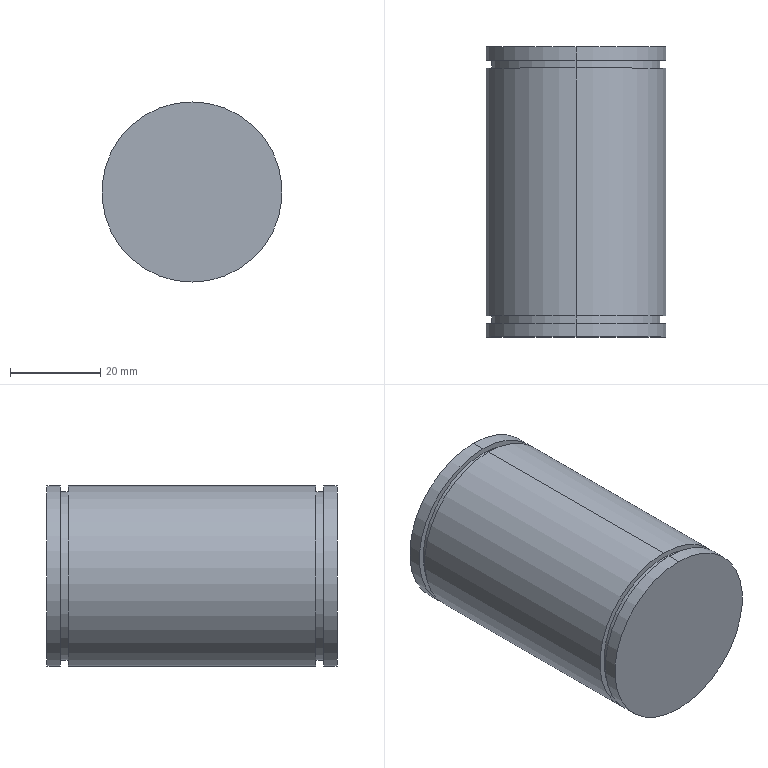Part | SolidWorks | features Extrusion 1, MirrorPattern 1, RevCut 1 | 1 solid | 16 faces | box 40 x 64.4 x 40 mm | volume 80410 mm3 | cylinder 10 | plane 6 | commonest cylinder face diameters 40 x6 37.5 x4
STEP:
#1=CARTESIAN_POINT('',(0.,3.,-20.));
#2=VERTEX_POINT('',#1);
#3=CARTESIAN_POINT('',(0.,3.,20.));
#4=VERTEX_POINT('',#3);
#5=CARTESIAN_POINT('',(0.,3.,0.));
#6=DIRECTION('',(0.,-1.,0.));
#7=DIRECTION('',(0.,0.,-1.));
#8=AXIS2_PLACEMENT_3D('',#5,#6,#7);
#9=CIRCLE('',#8,20.);
#10=EDGE_CURVE('',#2,#4,#9,.T.);
#11=ORIENTED_EDGE('',*,*,#10,.T.);
#12=CARTESIAN_POINT('',(0.,0.,20.));
#13=VERTEX_POINT('',#12);
#14=CARTESIAN_POINT('',(0.,64.4,20.));
#15=DIRECTION('',(0.,-1.,0.));
#16=VECTOR('',#15,1000.);
#17=LINE('',#14,#16);
#18=EDGE_CURVE('',#4,#13,#17,.T.);
#19=ORIENTED_EDGE('',*,*,#18,.T.);
#20=CARTESIAN_POINT('',(0.,0.,-20.));
#21=VERTEX_POINT('',#20);
#22=CARTESIAN_POINT('',(0.,0.,0.));
#23=DIRECTION('',(0.,1.,0.));
#24=DIRECTION('',(0.,0.,1.));
#25=AXIS2_PLACEMENT_3D('',#22,#23,#24);
#26=CIRCLE('',#25,20.);
#27=EDGE_CURVE('',#13,#21,#26,.T.);
#28=ORIENTED_EDGE('',*,*,#27,.T.);
#29=CARTESIAN_POINT('',(0.,64.4,-20.));
#30=DIRECTION('',(0.,-1.,0.));
#31=VECTOR('',#30,1000.);
#32=LINE('',#29,#31);
#33=EDGE_CURVE('',#2,#21,#32,.T.);
#34=ORIENTED_EDGE('',*,*,#33,.F.);
#35=EDGE_LOOP('',(#11,#19,#28,#34));
#36=FACE_OUTER_BOUND('',#35,.T.);
#37=CARTESIAN_POINT('',(0.,64.4,0.));
#38=DIRECTION('',(0.,-1.,0.));
#39=DIRECTION('',(0.,0.,-1.));
#40=AXIS2_PLACEMENT_3D('',#37,#38,#39);
#41=CYLINDRICAL_SURFACE('',#40,20.);
#42=ADVANCED_FACE('',(#36),#41,.T.);
#43=CARTESIAN_POINT('',(0.,4.7,-18.75));
#44=VERTEX_POINT('',#43);
#45=CARTESIAN_POINT('',(0.,4.7,18.75));
#46=VERTEX_POINT('',#45);
#47=CARTESIAN_POINT('',(0.,4.7,0.));
#48=DIRECTION('',(0.,1.,0.));
#49=DIRECTION('',(0.,0.,1.));
#50=AXIS2_PLACEMENT_3D('',#47,#48,#49);
#51=CIRCLE('',#50,18.75);
#52=EDGE_CURVE('',#44,#46,#51,.T.);
#53=ORIENTED_EDGE('',*,*,#52,.F.);
#54=CARTESIAN_POINT('',(0.,3.,-18.75));
#55=VERTEX_POINT('',#54);
#56=CARTESIAN_POINT('',(0.,0.,-18.75));
#57=DIRECTION('',(0.,-1.,0.));
#58=VECTOR('',#57,1000.);
#59=LINE('',#56,#58);
#60=EDGE_CURVE('',#44,#55,#59,.T.);
#61=ORIENTED_EDGE('',*,*,#60,.T.);
#62=CARTESIAN_POINT('',(0.,3.,18.75));
#63=VERTEX_POINT('',#62);
#64=CARTESIAN_POINT('',(0.,3.,0.));
#65=DIRECTION('',(0.,1.,0.));
#66=DIRECTION('',(0.,0.,1.));
#67=AXIS2_PLACEMENT_3D('',#64,#65,#66);
#68=CIRCLE('',#67,18.75);
#69=EDGE_CURVE('',#55,#63,#68,.T.);
#70=ORIENTED_EDGE('',*,*,#69,.T.);
#71=CARTESIAN_POINT('',(0.,0.,18.75));
#72=DIRECTION('',(0.,-1.,0.));
#73=VECTOR('',#72,1000.);
#74=LINE('',#71,#73);
#75=EDGE_CURVE('',#46,#63,#74,.T.);
#76=ORIENTED_EDGE('',*,*,#75,.F.);
#77=EDGE_LOOP('',(#53,#61,#70,#76));
#78=FACE_OUTER_BOUND('',#77,.T.);
#79=CARTESIAN_POINT('',(0.,0.,0.));
#80=DIRECTION('',(0.,-1.,0.));
#81=DIRECTION('',(0.,0.,1.));
#82=AXIS2_PLACEMENT_3D('',#79,#80,#81);
#83=CYLINDRICAL_SURFACE('',#82,18.75);
#84=ADVANCED_FACE('',(#78),#83,.T.);
#85=CARTESIAN_POINT('',(0.,64.4,20.));
#86=VERTEX_POINT('',#85);
#87=CARTESIAN_POINT('',(0.,64.4,-20.));
#88=VERTEX_POINT('',#87);
#89=CARTESIAN_POINT('',(0.,64.4,0.));
#90=DIRECTION('',(0.,1.,0.));
#91=DIRECTION('',(0.,0.,1.));
#92=AXIS2_PLACEMENT_3D('',#89,#90,#91);
#93=CIRCLE('',#92,20.);
#94=EDGE_CURVE('',#86,#88,#93,.T.);
#95=ORIENTED_EDGE('',*,*,#94,.F.);
#96=CARTESIAN_POINT('',(0.,61.4,20.));
#97=VERTEX_POINT('',#96);
#98=CARTESIAN_POINT('',(0.,64.4,20.));
#99=DIRECTION('',(0.,-1.,0.));
#100=VECTOR('',#99,1000.);
#101=LINE('',#98,#100);
#102=EDGE_CURVE('',#86,#97,#101,.T.);
#103=ORIENTED_EDGE('',*,*,#102,.T.);
#104=CARTESIAN_POINT('',(0.,61.4,-20.));
#105=VERTEX_POINT('',#104);
#106=CARTESIAN_POINT('',(0.,61.4,0.));
#107=DIRECTION('',(0.,1.,0.));
#108=DIRECTION('',(0.,0.,1.));
#109=AXIS2_PLACEMENT_3D('',#106,#107,#108);
#110=CIRCLE('',#109,20.);
#111=EDGE_CURVE('',#97,#105,#110,.T.);
#112=ORIENTED_EDGE('',*,*,#111,.T.);
#113=CARTESIAN_POINT('',(0.,64.4,-20.));
#114=DIRECTION('',(0.,-1.,0.));
#115=VECTOR('',#114,1000.);
#116=LINE('',#113,#115);
#117=EDGE_CURVE('',#88,#105,#116,.T.);
#118=ORIENTED_EDGE('',*,*,#117,.F.);
#119=EDGE_LOOP('',(#95,#103,#112,#118));
#120=FACE_OUTER_BOUND('',#119,.T.);
#121=CARTESIAN_POINT('',(0.,64.4,0.));
#122=DIRECTION('',(0.,-1.,0.));
#123=DIRECTION('',(0.,0.,-1.));
#124=AXIS2_PLACEMENT_3D('',#121,#122,#123);
#125=CYLINDRICAL_SURFACE('',#124,20.);
#126=ADVANCED_FACE('',(#120),#125,.T.);
#127=CARTESIAN_POINT('',(0.,59.7,18.75));
#128=VERTEX_POINT('',#127);
#129=CARTESIAN_POINT('',(0.,59.7,-18.75));
#130=VERTEX_POINT('',#129);
#131=CARTESIAN_POINT('',(0.,59.7,0.));
#132=DIRECTION('',(0.,1.,0.));
#133=DIRECTION('',(0.,0.,1.));
#134=AXIS2_PLACEMENT_3D('',#131,#132,#133);
#135=CIRCLE('',#134,18.75);
#136=EDGE_CURVE('',#128,#130,#135,.T.);
#137=ORIENTED_EDGE('',*,*,#136,.T.);
#138=CARTESIAN_POINT('',(0.,61.4,-18.75));
#139=VERTEX_POINT('',#138);
#140=CARTESIAN_POINT('',(0.,64.4,-18.75));
#141=DIRECTION('',(0.,1.,0.));
#142=VECTOR('',#141,1000.);
#143=LINE('',#140,#142);
#144=EDGE_CURVE('',#130,#139,#143,.T.);
#145=ORIENTED_EDGE('',*,*,#144,.T.);
#146=CARTESIAN_POINT('',(0.,61.4,18.75));
#147=VERTEX_POINT('',#146);
#148=CARTESIAN_POINT('',(0.,61.4,0.));
#149=DIRECTION('',(0.,1.,0.));
#150=DIRECTION('',(0.,0.,1.));
#151=AXIS2_PLACEMENT_3D('',#148,#149,#150);
#152=CIRCLE('',#151,18.75);
#153=EDGE_CURVE('',#147,#139,#152,.T.);
#154=ORIENTED_EDGE('',*,*,#153,.F.);
#155=CARTESIAN_POINT('',(0.,64.4,18.75));
#156=DIRECTION('',(0.,1.,0.));
#157=VECTOR('',#156,1000.);
#158=LINE('',#155,#157);
#159=EDGE_CURVE('',#128,#147,#158,.T.);
#160=ORIENTED_EDGE('',*,*,#159,.F.);
#161=EDGE_LOOP('',(#137,#145,#154,#160));
#162=FACE_OUTER_BOUND('',#161,.T.);
#163=CARTESIAN_POINT('',(0.,64.4,0.));
#164=DIRECTION('',(0.,1.,0.));
#165=DIRECTION('',(0.,0.,1.));
#166=AXIS2_PLACEMENT_3D('',#163,#164,#165);
#167=CYLINDRICAL_SURFACE('',#166,18.75);
#168=ADVANCED_FACE('',(#162),#167,.T.);
#169=CARTESIAN_POINT('',(0.,59.7,-20.));
#170=VERTEX_POINT('',#169);
#171=CARTESIAN_POINT('',(0.,59.7,20.));
#172=VERTEX_POINT('',#171);
#173=CARTESIAN_POINT('',(0.,59.7,0.));
#174=DIRECTION('',(0.,-1.,0.));
#175=DIRECTION('',(0.,0.,-1.));
#176=AXIS2_PLACEMENT_3D('',#173,#174,#175);
#177=CIRCLE('',#176,20.);
#178=EDGE_CURVE('',#170,#172,#177,.T.);
#179=ORIENTED_EDGE('',*,*,#178,.T.);
#180=CARTESIAN_POINT('',(0.,4.7,20.));
#181=VERTEX_POINT('',#180);
#182=CARTESIAN_POINT('',(0.,64.4,20.));
#183=DIRECTION('',(0.,-1.,0.));
#184=VECTOR('',#183,1000.);
#185=LINE('',#182,#184);
#186=EDGE_CURVE('',#172,#181,#185,.T.);
#187=ORIENTED_EDGE('',*,*,#186,.T.);
#188=CARTESIAN_POINT('',(0.,4.7,-20.));
#189=VERTEX_POINT('',#188);
#190=CARTESIAN_POINT('',(0.,4.7,0.));
#191=DIRECTION('',(0.,1.,0.));
#192=DIRECTION('',(0.,0.,1.));
#193=AXIS2_PLACEMENT_3D('',#190,#191,#192);
#194=CIRCLE('',#193,20.);
#195=EDGE_CURVE('',#181,#189,#194,.T.);
#196=ORIENTED_EDGE('',*,*,#195,.T.);
#197=CARTESIAN_POINT('',(0.,64.4,-20.));
#198=DIRECTION('',(0.,-1.,0.));
#199=VECTOR('',#198,1000.);
#200=LINE('',#197,#199);
#201=EDGE_CURVE('',#170,#189,#200,.T.);
#202=ORIENTED_EDGE('',*,*,#201,.F.);
#203=EDGE_LOOP('',(#179,#187,#196,#202));
#204=FACE_OUTER_BOUND('',#203,.T.);
#205=CARTESIAN_POINT('',(0.,64.4,0.));
#206=DIRECTION('',(0.,-1.,0.));
#207=DIRECTION('',(0.,0.,-1.));
#208=AXIS2_PLACEMENT_3D('',#205,#206,#207);
#209=CYLINDRICAL_SURFACE('',#208,20.);
#210=ADVANCED_FACE('',(#204),#209,.T.);
#211=ORIENTED_EDGE('',*,*,#186,.F.);
#212=CARTESIAN_POINT('',(0.,59.7,0.));
#213=DIRECTION('',(0.,-1.,0.));
#214=DIRECTION('',(0.,0.,-1.));
#215=AXIS2_PLACEMENT_3D('',#212,#213,#214);
#216=CIRCLE('',#215,20.);
#217=EDGE_CURVE('',#172,#170,#216,.T.);
#218=ORIENTED_EDGE('',*,*,#217,.T.);
#219=ORIENTED_EDGE('',*,*,#201,.T.);
#220=CARTESIAN_POINT('',(0.,4.7,0.));
#221=DIRECTION('',(0.,1.,0.));
#222=DIRECTION('',(0.,0.,1.));
#223=AXIS2_PLACEMENT_3D('',#220,#221,#222);
#224=CIRCLE('',#223,20.);
#225=EDGE_CURVE('',#189,#181,#224,.T.);
#226=ORIENTED_EDGE('',*,*,#225,.T.);
#227=EDGE_LOOP('',(#211,#218,#219,#226));
#228=FACE_OUTER_BOUND('',#227,.T.);
#229=CARTESIAN_POINT('',(0.,64.4,0.));
#230=DIRECTION('',(0.,-1.,0.));
#231=DIRECTION('',(0.,0.,-1.));
#232=AXIS2_PLACEMENT_3D('',#229,#230,#231);
#233=CYLINDRICAL_SURFACE('',#232,20.);
#234=ADVANCED_FACE('',(#228),#233,.T.);
#235=ORIENTED_EDGE('',*,*,#136,.F.);
#236=CARTESIAN_POINT('',(0.,59.7,0.));
#237=DIRECTION('',(0.,1.,0.));
#238=DIRECTION('',(0.,0.,1.));
#239=AXIS2_PLACEMENT_3D('',#236,#237,#238);
#240=CIRCLE('',#239,18.75);
#241=EDGE_CURVE('',#130,#128,#240,.T.);
#242=ORIENTED_EDGE('',*,*,#241,.F.);
#243=EDGE_LOOP('',(#235,#242));
#244=FACE_BOUND('',#243,.T.);
#245=ORIENTED_EDGE('',*,*,#178,.F.);
#246=ORIENTED_EDGE('',*,*,#217,.F.);
#247=EDGE_LOOP('',(#245,#246));
#248=FACE_OUTER_BOUND('',#247,.T.);
#249=CARTESIAN_POINT('',(-22.076,59.7,0.));
#250=DIRECTION('',(0.,-1.,0.));
#251=DIRECTION('',(0.,0.,-1.));
#252=AXIS2_PLACEMENT_3D('',#249,#250,#251);
#253=PLANE('',#252);
#254=ADVANCED_FACE('',(#244,#248),#253,.F.);
#255=ORIENTED_EDGE('',*,*,#153,.T.);
#256=CARTESIAN_POINT('',(0.,61.4,0.));
#257=DIRECTION('',(0.,1.,0.));
#258=DIRECTION('',(0.,0.,1.));
#259=AXIS2_PLACEMENT_3D('',#256,#257,#258);
#260=CIRCLE('',#259,18.75);
#261=EDGE_CURVE('',#139,#147,#260,.T.);
#262=ORIENTED_EDGE('',*,*,#261,.T.);
#263=EDGE_LOOP('',(#255,#262));
#264=FACE_BOUND('',#263,.T.);
#265=CARTESIAN_POINT('',(0.,61.4,0.));
#266=DIRECTION('',(0.,1.,0.));
#267=DIRECTION('',(0.,0.,1.));
#268=AXIS2_PLACEMENT_3D('',#265,#266,#267);
#269=CIRCLE('',#268,20.);
#270=EDGE_CURVE('',#105,#97,#269,.T.);
#271=ORIENTED_EDGE('',*,*,#270,.F.);
#272=ORIENTED_EDGE('',*,*,#111,.F.);
#273=EDGE_LOOP('',(#271,#272));
#274=FACE_OUTER_BOUND('',#273,.T.);
#275=CARTESIAN_POINT('',(-22.076,61.4,0.));
#276=DIRECTION('',(0.,1.,0.));
#277=DIRECTION('',(0.,0.,1.));
#278=AXIS2_PLACEMENT_3D('',#275,#276,#277);
#279=PLANE('',#278);
#280=ADVANCED_FACE('',(#264,#274),#279,.F.);
#281=ORIENTED_EDGE('',*,*,#144,.F.);
#282=ORIENTED_EDGE('',*,*,#241,.T.);
#283=ORIENTED_EDGE('',*,*,#159,.T.);
#284=ORIENTED_EDGE('',*,*,#261,.F.);
#285=EDGE_LOOP('',(#281,#282,#283,#284));
#286=FACE_OUTER_BOUND('',#285,.T.);
#287=CARTESIAN_POINT('',(0.,64.4,0.));
#288=DIRECTION('',(0.,1.,0.));
#289=DIRECTION('',(0.,0.,1.));
#290=AXIS2_PLACEMENT_3D('',#287,#288,#289);
#291=CYLINDRICAL_SURFACE('',#290,18.75);
#292=ADVANCED_FACE('',(#286),#291,.T.);
#293=CARTESIAN_POINT('',(0.,64.4,0.));
#294=DIRECTION('',(0.,1.,0.));
#295=DIRECTION('',(0.,0.,1.));
#296=AXIS2_PLACEMENT_3D('',#293,#294,#295);
#297=CIRCLE('',#296,20.);
#298=EDGE_CURVE('',#88,#86,#297,.T.);
#299=ORIENTED_EDGE('',*,*,#298,.T.);
#300=ORIENTED_EDGE('',*,*,#94,.T.);
#301=EDGE_LOOP('',(#299,#300));
#302=FACE_OUTER_BOUND('',#301,.T.);
#303=CARTESIAN_POINT('',(0.,64.4,0.));
#304=DIRECTION('',(0.,1.,0.));
#305=DIRECTION('',(0.,0.,1.));
#306=AXIS2_PLACEMENT_3D('',#303,#304,#305);
#307=PLANE('',#306);
#308=ADVANCED_FACE('',(#302),#307,.T.);
#309=ORIENTED_EDGE('',*,*,#102,.F.);
#310=ORIENTED_EDGE('',*,*,#298,.F.);
#311=ORIENTED_EDGE('',*,*,#117,.T.);
#312=ORIENTED_EDGE('',*,*,#270,.T.);
#313=EDGE_LOOP('',(#309,#310,#311,#312));
#314=FACE_OUTER_BOUND('',#313,.T.);
#315=CARTESIAN_POINT('',(0.,64.4,0.));
#316=DIRECTION('',(0.,-1.,0.));
#317=DIRECTION('',(0.,0.,-1.));
#318=AXIS2_PLACEMENT_3D('',#315,#316,#317);
#319=CYLINDRICAL_SURFACE('',#318,20.);
#320=ADVANCED_FACE('',(#314),#319,.T.);
#321=CARTESIAN_POINT('',(0.,4.7,0.));
#322=DIRECTION('',(0.,1.,0.));
#323=DIRECTION('',(0.,0.,1.));
#324=AXIS2_PLACEMENT_3D('',#321,#322,#323);
#325=CIRCLE('',#324,18.75);
#326=EDGE_CURVE('',#46,#44,#325,.T.);
#327=ORIENTED_EDGE('',*,*,#326,.T.);
#328=ORIENTED_EDGE('',*,*,#52,.T.);
#329=EDGE_LOOP('',(#327,#328));
#330=FACE_BOUND('',#329,.T.);
#331=ORIENTED_EDGE('',*,*,#225,.F.);
#332=ORIENTED_EDGE('',*,*,#195,.F.);
#333=EDGE_LOOP('',(#331,#332));
#334=FACE_OUTER_BOUND('',#333,.T.);
#335=CARTESIAN_POINT('',(-22.076,4.7,0.));
#336=DIRECTION('',(0.,1.,0.));
#337=DIRECTION('',(0.,0.,-1.));
#338=AXIS2_PLACEMENT_3D('',#335,#336,#337);
#339=PLANE('',#338);
#340=ADVANCED_FACE('',(#330,#334),#339,.F.);
#341=CARTESIAN_POINT('',(0.,3.,0.));
#342=DIRECTION('',(0.,1.,0.));
#343=DIRECTION('',(0.,0.,1.));
#344=AXIS2_PLACEMENT_3D('',#341,#342,#343);
#345=CIRCLE('',#344,18.75);
#346=EDGE_CURVE('',#63,#55,#345,.T.);
#347=ORIENTED_EDGE('',*,*,#346,.F.);
#348=ORIENTED_EDGE('',*,*,#69,.F.);
#349=EDGE_LOOP('',(#347,#348));
#350=FACE_BOUND('',#349,.T.);
#351=ORIENTED_EDGE('',*,*,#10,.F.);
#352=CARTESIAN_POINT('',(0.,3.,0.));
#353=DIRECTION('',(0.,-1.,0.));
#354=DIRECTION('',(0.,0.,-1.));
#355=AXIS2_PLACEMENT_3D('',#352,#353,#354);
#356=CIRCLE('',#355,20.);
#357=EDGE_CURVE('',#4,#2,#356,.T.);
#358=ORIENTED_EDGE('',*,*,#357,.F.);
#359=EDGE_LOOP('',(#351,#358));
#360=FACE_OUTER_BOUND('',#359,.T.);
#361=CARTESIAN_POINT('',(-22.076,3.,0.));
#362=DIRECTION('',(0.,-1.,0.));
#363=DIRECTION('',(0.,0.,1.));
#364=AXIS2_PLACEMENT_3D('',#361,#362,#363);
#365=PLANE('',#364);
#366=ADVANCED_FACE('',(#350,#360),#365,.F.);
#367=ORIENTED_EDGE('',*,*,#60,.F.);
#368=ORIENTED_EDGE('',*,*,#326,.F.);
#369=ORIENTED_EDGE('',*,*,#75,.T.);
#370=ORIENTED_EDGE('',*,*,#346,.T.);
#371=EDGE_LOOP('',(#367,#368,#369,#370));
#372=FACE_OUTER_BOUND('',#371,.T.);
#373=CARTESIAN_POINT('',(0.,0.,0.));
#374=DIRECTION('',(0.,-1.,0.));
#375=DIRECTION('',(0.,0.,1.));
#376=AXIS2_PLACEMENT_3D('',#373,#374,#375);
#377=CYLINDRICAL_SURFACE('',#376,18.75);
#378=ADVANCED_FACE('',(#372),#377,.T.);
#379=CARTESIAN_POINT('',(0.,0.,0.));
#380=DIRECTION('',(0.,1.,0.));
#381=DIRECTION('',(0.,0.,1.));
#382=AXIS2_PLACEMENT_3D('',#379,#380,#381);
#383=CIRCLE('',#382,20.);
#384=EDGE_CURVE('',#21,#13,#383,.T.);
#385=ORIENTED_EDGE('',*,*,#384,.F.);
#386=ORIENTED_EDGE('',*,*,#27,.F.);
#387=EDGE_LOOP('',(#385,#386));
#388=FACE_OUTER_BOUND('',#387,.T.);
#389=CARTESIAN_POINT('',(0.,0.,0.));
#390=DIRECTION('',(0.,1.,0.));
#391=DIRECTION('',(0.,0.,1.));
#392=AXIS2_PLACEMENT_3D('',#389,#390,#391);
#393=PLANE('',#392);
#394=ADVANCED_FACE('',(#388),#393,.F.);
#395=ORIENTED_EDGE('',*,*,#18,.F.);
#396=ORIENTED_EDGE('',*,*,#357,.T.);
#397=ORIENTED_EDGE('',*,*,#33,.T.);
#398=ORIENTED_EDGE('',*,*,#384,.T.);
#399=EDGE_LOOP('',(#395,#396,#397,#398));
#400=FACE_OUTER_BOUND('',#399,.T.);
#401=CARTESIAN_POINT('',(0.,64.4,0.));
#402=DIRECTION('',(0.,-1.,0.));
#403=DIRECTION('',(0.,0.,-1.));
#404=AXIS2_PLACEMENT_3D('',#401,#402,#403);
#405=CYLINDRICAL_SURFACE('',#404,20.);
#406=ADVANCED_FACE('',(#400),#405,.T.);
#407=CLOSED_SHELL('',(#42,#84,#126,#168,#210,#234,#254,#280,#292,#308,#320,#340,#366,#378,#394,#406));
#408=MANIFOLD_SOLID_BREP('',#407);
#409=CARTESIAN_POINT('',(0.,0.,0.));
#410=DIRECTION('',(0.,0.,1.));
#411=DIRECTION('',(1.,0.,0.));
#412=AXIS2_PLACEMENT_3D('',#409,#410,#411);
#413=(LENGTH_UNIT()NAMED_UNIT(*)SI_UNIT(.MILLI.,.METRE.));
#414=UNCERTAINTY_MEASURE_WITH_UNIT(LENGTH_MEASURE(0.00001),#413,'','');
#415=(NAMED_UNIT(*)PLANE_ANGLE_UNIT()SI_UNIT($,.RADIAN.));
#416=(NAMED_UNIT(*)SI_UNIT($,.STERADIAN.)SOLID_ANGLE_UNIT());
#417=(GEOMETRIC_REPRESENTATION_CONTEXT(3)GLOBAL_UNCERTAINTY_ASSIGNED_CONTEXT((#414))GLOBAL_UNIT_ASSIGNED_CONTEXT((#413,#415,#416))REPRESENTATION_CONTEXT('',''));
#418=ADVANCED_BREP_SHAPE_REPRESENTATION('',(#408,#412),#417);